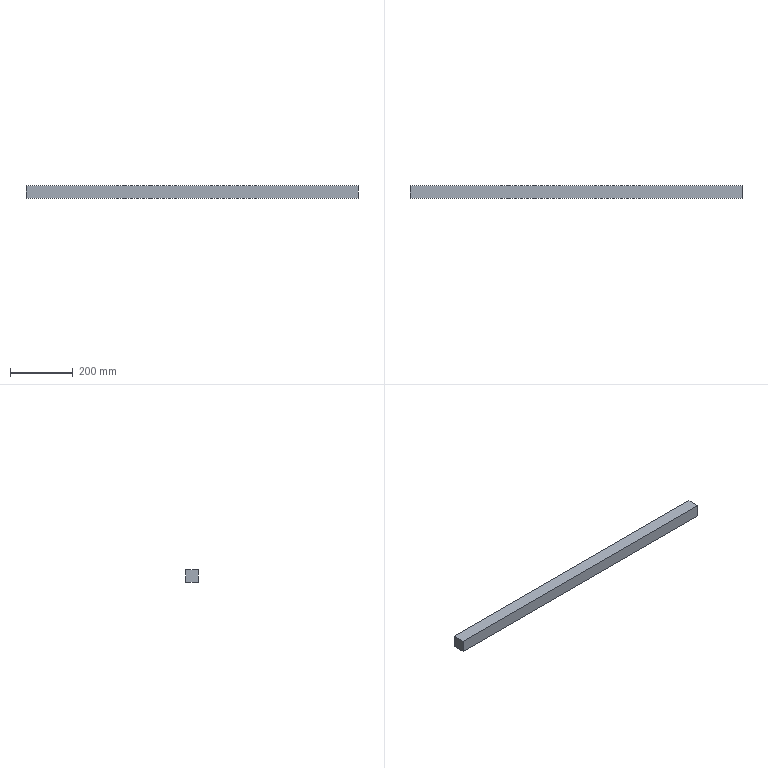Part | NX | features 凸台-拉伸19 2 | 1 solid | 6 faces | box 1060 x 40 x 40 mm | volume 1696000 mm3 | plane 6
STEP:
#1=CARTESIAN_POINT('',(-127.,-560.,-212.985));
#2=VERTEX_POINT('',#1);
#3=CARTESIAN_POINT('',(-127.,-560.,-252.985));
#4=VERTEX_POINT('',#3);
#5=CARTESIAN_POINT('',(-127.,-560.,-252.985));
#6=DIRECTION('',(0.,0.,-1.));
#7=VECTOR('',#6,1000.);
#8=LINE('',#5,#7);
#9=EDGE_CURVE('',#2,#4,#8,.T.);
#10=ORIENTED_EDGE('',*,*,#9,.T.);
#11=CARTESIAN_POINT('',(-127.,-600.,-252.985));
#12=VERTEX_POINT('',#11);
#13=CARTESIAN_POINT('',(-127.,-560.,-252.985));
#14=DIRECTION('',(0.,-1.,0.));
#15=VECTOR('',#14,1000.);
#16=LINE('',#13,#15);
#17=EDGE_CURVE('',#4,#12,#16,.T.);
#18=ORIENTED_EDGE('',*,*,#17,.T.);
#19=CARTESIAN_POINT('',(-127.,-600.,-212.985));
#20=VERTEX_POINT('',#19);
#21=CARTESIAN_POINT('',(-127.,-600.,-252.985));
#22=DIRECTION('',(0.,0.,1.));
#23=VECTOR('',#22,1000.);
#24=LINE('',#21,#23);
#25=EDGE_CURVE('',#12,#20,#24,.T.);
#26=ORIENTED_EDGE('',*,*,#25,.T.);
#27=CARTESIAN_POINT('',(-127.,-560.,-212.985));
#28=DIRECTION('',(0.,1.,0.));
#29=VECTOR('',#28,1000.);
#30=LINE('',#27,#29);
#31=EDGE_CURVE('',#20,#2,#30,.T.);
#32=ORIENTED_EDGE('',*,*,#31,.T.);
#33=EDGE_LOOP('',(#10,#18,#26,#32));
#34=FACE_BOUND('',#33,.T.);
#35=CARTESIAN_POINT('',(-127.,-600.,-1389.553));
#36=DIRECTION('',(-1.,0.,0.));
#37=DIRECTION('',(0.,0.,1.));
#38=AXIS2_PLACEMENT_3D('',#35,#36,#37);
#39=PLANE('',#38);
#40=ADVANCED_FACE('',(#34),#39,.T.);
#41=CARTESIAN_POINT('',(933.,-560.,-252.985));
#42=VERTEX_POINT('',#41);
#43=CARTESIAN_POINT('',(933.,-600.,-252.985));
#44=VERTEX_POINT('',#43);
#45=CARTESIAN_POINT('',(933.,-560.,-252.985));
#46=DIRECTION('',(0.,-1.,0.));
#47=VECTOR('',#46,1000.);
#48=LINE('',#45,#47);
#49=EDGE_CURVE('',#42,#44,#48,.T.);
#50=ORIENTED_EDGE('',*,*,#49,.F.);
#51=CARTESIAN_POINT('',(933.,-560.,-212.985));
#52=VERTEX_POINT('',#51);
#53=CARTESIAN_POINT('',(933.,-560.,-252.985));
#54=DIRECTION('',(0.,0.,-1.));
#55=VECTOR('',#54,1000.);
#56=LINE('',#53,#55);
#57=EDGE_CURVE('',#52,#42,#56,.T.);
#58=ORIENTED_EDGE('',*,*,#57,.F.);
#59=CARTESIAN_POINT('',(933.,-600.,-212.985));
#60=VERTEX_POINT('',#59);
#61=CARTESIAN_POINT('',(933.,-560.,-212.985));
#62=DIRECTION('',(0.,1.,0.));
#63=VECTOR('',#62,1000.);
#64=LINE('',#61,#63);
#65=EDGE_CURVE('',#60,#52,#64,.T.);
#66=ORIENTED_EDGE('',*,*,#65,.F.);
#67=CARTESIAN_POINT('',(933.,-600.,-252.985));
#68=DIRECTION('',(0.,0.,1.));
#69=VECTOR('',#68,1000.);
#70=LINE('',#67,#69);
#71=EDGE_CURVE('',#44,#60,#70,.T.);
#72=ORIENTED_EDGE('',*,*,#71,.F.);
#73=EDGE_LOOP('',(#50,#58,#66,#72));
#74=FACE_BOUND('',#73,.T.);
#75=CARTESIAN_POINT('',(933.,0.,0.));
#76=DIRECTION('',(-1.,0.,0.));
#77=DIRECTION('',(0.,0.,1.));
#78=AXIS2_PLACEMENT_3D('',#75,#76,#77);
#79=PLANE('',#78);
#80=ADVANCED_FACE('',(#74),#79,.F.);
#81=ORIENTED_EDGE('',*,*,#9,.F.);
#82=CARTESIAN_POINT('',(-183.569,-560.,-212.985));
#83=DIRECTION('',(1.,0.,0.));
#84=VECTOR('',#83,1000.);
#85=LINE('',#82,#84);
#86=EDGE_CURVE('',#2,#52,#85,.T.);
#87=ORIENTED_EDGE('',*,*,#86,.T.);
#88=ORIENTED_EDGE('',*,*,#57,.T.);
#89=CARTESIAN_POINT('',(-183.569,-560.,-252.985));
#90=DIRECTION('',(1.,0.,0.));
#91=VECTOR('',#90,1000.);
#92=LINE('',#89,#91);
#93=EDGE_CURVE('',#4,#42,#92,.T.);
#94=ORIENTED_EDGE('',*,*,#93,.F.);
#95=EDGE_LOOP('',(#81,#87,#88,#94));
#96=FACE_BOUND('',#95,.T.);
#97=CARTESIAN_POINT('',(-183.569,-560.,-252.985));
#98=DIRECTION('',(0.,-1.,0.));
#99=DIRECTION('',(0.,0.,-1.));
#100=AXIS2_PLACEMENT_3D('',#97,#98,#99);
#101=PLANE('',#100);
#102=ADVANCED_FACE('',(#96),#101,.F.);
#103=ORIENTED_EDGE('',*,*,#31,.F.);
#104=CARTESIAN_POINT('',(-183.569,-600.,-212.985));
#105=DIRECTION('',(1.,0.,0.));
#106=VECTOR('',#105,1000.);
#107=LINE('',#104,#106);
#108=EDGE_CURVE('',#20,#60,#107,.T.);
#109=ORIENTED_EDGE('',*,*,#108,.T.);
#110=ORIENTED_EDGE('',*,*,#65,.T.);
#111=ORIENTED_EDGE('',*,*,#86,.F.);
#112=EDGE_LOOP('',(#103,#109,#110,#111));
#113=FACE_BOUND('',#112,.T.);
#114=CARTESIAN_POINT('',(-183.569,-560.,-212.985));
#115=DIRECTION('',(0.,0.,-1.));
#116=DIRECTION('',(-1.,0.,0.));
#117=AXIS2_PLACEMENT_3D('',#114,#115,#116);
#118=PLANE('',#117);
#119=ADVANCED_FACE('',(#113),#118,.F.);
#120=ORIENTED_EDGE('',*,*,#25,.F.);
#121=CARTESIAN_POINT('',(-183.569,-600.,-252.985));
#122=DIRECTION('',(1.,0.,0.));
#123=VECTOR('',#122,1000.);
#124=LINE('',#121,#123);
#125=EDGE_CURVE('',#12,#44,#124,.T.);
#126=ORIENTED_EDGE('',*,*,#125,.T.);
#127=ORIENTED_EDGE('',*,*,#71,.T.);
#128=ORIENTED_EDGE('',*,*,#108,.F.);
#129=EDGE_LOOP('',(#120,#126,#127,#128));
#130=FACE_BOUND('',#129,.T.);
#131=CARTESIAN_POINT('',(-183.569,-600.,-252.985));
#132=DIRECTION('',(0.,1.,0.));
#133=DIRECTION('',(0.,0.,1.));
#134=AXIS2_PLACEMENT_3D('',#131,#132,#133);
#135=PLANE('',#134);
#136=ADVANCED_FACE('',(#130),#135,.F.);
#137=ORIENTED_EDGE('',*,*,#17,.F.);
#138=ORIENTED_EDGE('',*,*,#93,.T.);
#139=ORIENTED_EDGE('',*,*,#49,.T.);
#140=ORIENTED_EDGE('',*,*,#125,.F.);
#141=EDGE_LOOP('',(#137,#138,#139,#140));
#142=FACE_BOUND('',#141,.T.);
#143=CARTESIAN_POINT('',(-183.569,-560.,-252.985));
#144=DIRECTION('',(0.,0.,1.));
#145=DIRECTION('',(1.,0.,0.));
#146=AXIS2_PLACEMENT_3D('',#143,#144,#145);
#147=PLANE('',#146);
#148=ADVANCED_FACE('',(#142),#147,.F.);
#149=CLOSED_SHELL('',(#40,#80,#102,#119,#136,#148));
#150=MANIFOLD_SOLID_BREP('',#149);
#151=(LENGTH_UNIT()NAMED_UNIT(*)SI_UNIT(.MILLI.,.METRE.));
#152=UNCERTAINTY_MEASURE_WITH_UNIT(LENGTH_MEASURE(0.00001),#151,'','');
#153=(NAMED_UNIT(*)PLANE_ANGLE_UNIT()SI_UNIT($,.RADIAN.));
#154=(NAMED_UNIT(*)SI_UNIT($,.STERADIAN.)SOLID_ANGLE_UNIT());
#155=(GEOMETRIC_REPRESENTATION_CONTEXT(3)GLOBAL_UNCERTAINTY_ASSIGNED_CONTEXT((#152))GLOBAL_UNIT_ASSIGNED_CONTEXT((#151,#153,#154))REPRESENTATION_CONTEXT('',''));
#156=ADVANCED_BREP_SHAPE_REPRESENTATION('',(#150),#155);